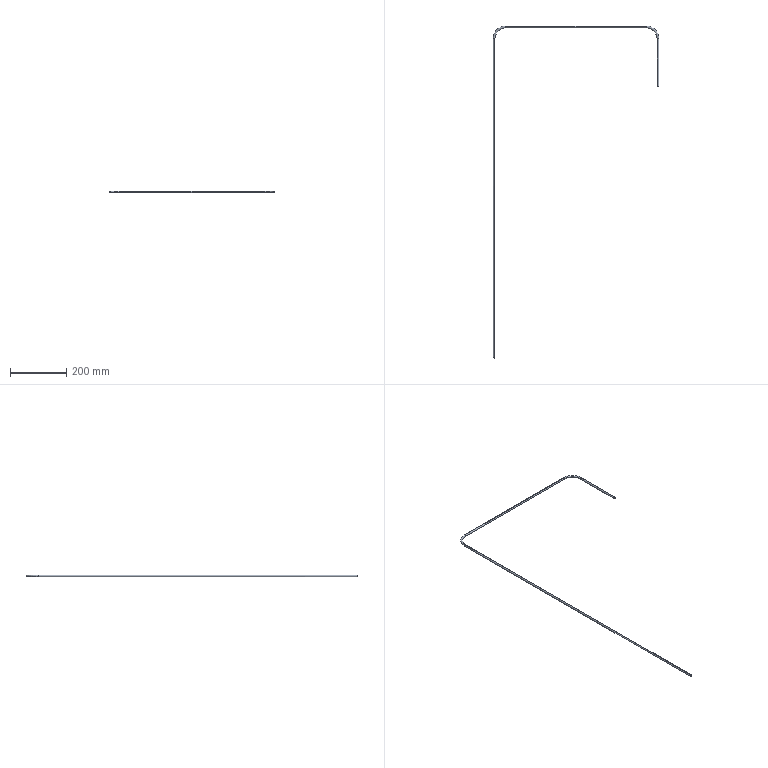Part | SolidWorks | features Sweep 1 | 1 solid | 12 faces | box 588.5 x 1178 x 6.5 mm | volume 64106 mm3 | cylinder 6 | torus 4 | plane 2 | commonest cylinder face diameters 6.5 x6
STEP:
#1=CARTESIAN_POINT('',(540.,1175.,-3.25));
#2=VERTEX_POINT('',#1);
#3=CARTESIAN_POINT('',(540.,1178.25,0.));
#4=VERTEX_POINT('',#3);
#5=CARTESIAN_POINT('',(540.,1175.,0.));
#6=DIRECTION('',(1.,0.,0.));
#7=DIRECTION('',(0.,0.,1.));
#8=AXIS2_PLACEMENT_3D('',#5,#6,#7);
#9=CIRCLE('',#8,3.25);
#10=EDGE_CURVE('',#2,#4,#9,.T.);
#11=ORIENTED_EDGE('',*,*,#10,.T.);
#12=CARTESIAN_POINT('',(585.25,1133.,0.));
#13=VERTEX_POINT('',#12);
#14=CARTESIAN_POINT('',(540.,1133.,0.));
#15=DIRECTION('',(0.,0.,-1.));
#16=DIRECTION('',(-1.,0.,0.));
#17=AXIS2_PLACEMENT_3D('',#14,#15,#16);
#18=CIRCLE('',#17,45.25);
#19=EDGE_CURVE('',#4,#13,#18,.T.);
#20=ORIENTED_EDGE('',*,*,#19,.T.);
#21=CARTESIAN_POINT('',(582.,1133.,-3.25));
#22=VERTEX_POINT('',#21);
#23=CARTESIAN_POINT('',(582.,1133.,0.));
#24=DIRECTION('',(0.,-1.,0.));
#25=DIRECTION('',(0.,0.,1.));
#26=AXIS2_PLACEMENT_3D('',#23,#24,#25);
#27=CIRCLE('',#26,3.25);
#28=EDGE_CURVE('',#22,#13,#27,.T.);
#29=ORIENTED_EDGE('',*,*,#28,.F.);
#30=CARTESIAN_POINT('',(578.75,1133.,0.));
#31=VERTEX_POINT('',#30);
#32=CARTESIAN_POINT('',(582.,1133.,0.));
#33=DIRECTION('',(0.,-1.,0.));
#34=DIRECTION('',(0.,0.,1.));
#35=AXIS2_PLACEMENT_3D('',#32,#33,#34);
#36=CIRCLE('',#35,3.25);
#37=EDGE_CURVE('',#31,#22,#36,.T.);
#38=ORIENTED_EDGE('',*,*,#37,.F.);
#39=CARTESIAN_POINT('',(540.,1171.75,0.));
#40=VERTEX_POINT('',#39);
#41=CARTESIAN_POINT('',(540.,1133.,0.));
#42=DIRECTION('',(0.,0.,-1.));
#43=DIRECTION('',(-1.,0.,0.));
#44=AXIS2_PLACEMENT_3D('',#41,#42,#43);
#45=CIRCLE('',#44,38.75);
#46=EDGE_CURVE('',#40,#31,#45,.T.);
#47=ORIENTED_EDGE('',*,*,#46,.F.);
#48=CARTESIAN_POINT('',(540.,1175.,0.));
#49=DIRECTION('',(1.,0.,0.));
#50=DIRECTION('',(0.,0.,1.));
#51=AXIS2_PLACEMENT_3D('',#48,#49,#50);
#52=CIRCLE('',#51,3.25);
#53=EDGE_CURVE('',#40,#2,#52,.T.);
#54=ORIENTED_EDGE('',*,*,#53,.T.);
#55=EDGE_LOOP('',(#11,#20,#29,#38,#47,#54));
#56=FACE_OUTER_BOUND('',#55,.T.);
#57=CARTESIAN_POINT('',(540.,1133.,0.));
#58=DIRECTION('',(0.,0.,-1.));
#59=DIRECTION('',(-1.,0.,0.));
#60=AXIS2_PLACEMENT_3D('',#57,#58,#59);
#61=TOROIDAL_SURFACE('',#60,42.,3.25);
#62=ADVANCED_FACE('',(#56),#61,.T.);
#63=CARTESIAN_POINT('',(0.,1133.,-3.25));
#64=VERTEX_POINT('',#63);
#65=CARTESIAN_POINT('',(-3.25,1133.,0.));
#66=VERTEX_POINT('',#65);
#67=CARTESIAN_POINT('',(0.,1133.,0.));
#68=DIRECTION('',(0.,1.,0.));
#69=DIRECTION('',(0.,0.,1.));
#70=AXIS2_PLACEMENT_3D('',#67,#68,#69);
#71=CIRCLE('',#70,3.25);
#72=EDGE_CURVE('',#64,#66,#71,.T.);
#73=ORIENTED_EDGE('',*,*,#72,.T.);
#74=CARTESIAN_POINT('',(42.,1178.25,0.));
#75=VERTEX_POINT('',#74);
#76=CARTESIAN_POINT('',(42.,1133.,0.));
#77=DIRECTION('',(0.,0.,-1.));
#78=DIRECTION('',(-1.,0.,0.));
#79=AXIS2_PLACEMENT_3D('',#76,#77,#78);
#80=CIRCLE('',#79,45.25);
#81=EDGE_CURVE('',#66,#75,#80,.T.);
#82=ORIENTED_EDGE('',*,*,#81,.T.);
#83=CARTESIAN_POINT('',(42.,1175.,-3.25));
#84=VERTEX_POINT('',#83);
#85=CARTESIAN_POINT('',(42.,1175.,0.));
#86=DIRECTION('',(1.,0.,0.));
#87=DIRECTION('',(0.,0.,1.));
#88=AXIS2_PLACEMENT_3D('',#85,#86,#87);
#89=CIRCLE('',#88,3.25);
#90=EDGE_CURVE('',#84,#75,#89,.T.);
#91=ORIENTED_EDGE('',*,*,#90,.F.);
#92=CARTESIAN_POINT('',(42.,1171.75,0.));
#93=VERTEX_POINT('',#92);
#94=CARTESIAN_POINT('',(42.,1175.,0.));
#95=DIRECTION('',(1.,0.,0.));
#96=DIRECTION('',(0.,0.,1.));
#97=AXIS2_PLACEMENT_3D('',#94,#95,#96);
#98=CIRCLE('',#97,3.25);
#99=EDGE_CURVE('',#93,#84,#98,.T.);
#100=ORIENTED_EDGE('',*,*,#99,.F.);
#101=CARTESIAN_POINT('',(3.25,1133.,0.));
#102=VERTEX_POINT('',#101);
#103=CARTESIAN_POINT('',(42.,1133.,0.));
#104=DIRECTION('',(0.,0.,-1.));
#105=DIRECTION('',(-1.,0.,0.));
#106=AXIS2_PLACEMENT_3D('',#103,#104,#105);
#107=CIRCLE('',#106,38.75);
#108=EDGE_CURVE('',#102,#93,#107,.T.);
#109=ORIENTED_EDGE('',*,*,#108,.F.);
#110=CARTESIAN_POINT('',(0.,1133.,0.));
#111=DIRECTION('',(0.,1.,0.));
#112=DIRECTION('',(0.,0.,1.));
#113=AXIS2_PLACEMENT_3D('',#110,#111,#112);
#114=CIRCLE('',#113,3.25);
#115=EDGE_CURVE('',#102,#64,#114,.T.);
#116=ORIENTED_EDGE('',*,*,#115,.T.);
#117=EDGE_LOOP('',(#73,#82,#91,#100,#109,#116));
#118=FACE_OUTER_BOUND('',#117,.T.);
#119=CARTESIAN_POINT('',(42.,1133.,0.));
#120=DIRECTION('',(0.,0.,-1.));
#121=DIRECTION('',(-1.,0.,0.));
#122=AXIS2_PLACEMENT_3D('',#119,#120,#121);
#123=TOROIDAL_SURFACE('',#122,42.,3.25);
#124=ADVANCED_FACE('',(#118),#123,.T.);
#125=ORIENTED_EDGE('',*,*,#28,.T.);
#126=CARTESIAN_POINT('',(582.,1133.,3.25));
#127=VERTEX_POINT('',#126);
#128=CARTESIAN_POINT('',(582.,1133.,0.));
#129=DIRECTION('',(0.,-1.,0.));
#130=DIRECTION('',(0.,0.,1.));
#131=AXIS2_PLACEMENT_3D('',#128,#129,#130);
#132=CIRCLE('',#131,3.25);
#133=EDGE_CURVE('',#13,#127,#132,.T.);
#134=ORIENTED_EDGE('',*,*,#133,.T.);
#135=CARTESIAN_POINT('',(582.,964.057,3.25));
#136=VERTEX_POINT('',#135);
#137=CARTESIAN_POINT('',(582.,1133.,3.25));
#138=DIRECTION('',(0.,-1.,0.));
#139=VECTOR('',#138,1000.);
#140=LINE('',#137,#139);
#141=EDGE_CURVE('',#127,#136,#140,.T.);
#142=ORIENTED_EDGE('',*,*,#141,.T.);
#143=CARTESIAN_POINT('',(582.,964.057,-3.25));
#144=VERTEX_POINT('',#143);
#145=CARTESIAN_POINT('',(582.,964.057,0.));
#146=DIRECTION('',(0.,-1.,0.));
#147=DIRECTION('',(0.,0.,1.));
#148=AXIS2_PLACEMENT_3D('',#145,#146,#147);
#149=CIRCLE('',#148,3.25);
#150=EDGE_CURVE('',#144,#136,#149,.T.);
#151=ORIENTED_EDGE('',*,*,#150,.F.);
#152=CARTESIAN_POINT('',(582.,1133.,-3.25));
#153=DIRECTION('',(0.,-1.,0.));
#154=VECTOR('',#153,1000.);
#155=LINE('',#152,#154);
#156=EDGE_CURVE('',#22,#144,#155,.T.);
#157=ORIENTED_EDGE('',*,*,#156,.F.);
#158=EDGE_LOOP('',(#125,#134,#142,#151,#157));
#159=FACE_OUTER_BOUND('',#158,.T.);
#160=CARTESIAN_POINT('',(582.,1133.,0.));
#161=DIRECTION('',(0.,-1.,0.));
#162=DIRECTION('',(0.,0.,-1.));
#163=AXIS2_PLACEMENT_3D('',#160,#161,#162);
#164=CYLINDRICAL_SURFACE('',#163,3.25);
#165=ADVANCED_FACE('',(#159),#164,.T.);
#166=ORIENTED_EDGE('',*,*,#90,.T.);
#167=CARTESIAN_POINT('',(42.,1175.,3.25));
#168=VERTEX_POINT('',#167);
#169=CARTESIAN_POINT('',(42.,1175.,0.));
#170=DIRECTION('',(1.,0.,0.));
#171=DIRECTION('',(0.,0.,1.));
#172=AXIS2_PLACEMENT_3D('',#169,#170,#171);
#173=CIRCLE('',#172,3.25);
#174=EDGE_CURVE('',#75,#168,#173,.T.);
#175=ORIENTED_EDGE('',*,*,#174,.T.);
#176=CARTESIAN_POINT('',(540.,1175.,3.25));
#177=VERTEX_POINT('',#176);
#178=CARTESIAN_POINT('',(42.,1175.,3.25));
#179=DIRECTION('',(1.,0.,0.));
#180=VECTOR('',#179,1000.);
#181=LINE('',#178,#180);
#182=EDGE_CURVE('',#168,#177,#181,.T.);
#183=ORIENTED_EDGE('',*,*,#182,.T.);
#184=CARTESIAN_POINT('',(540.,1175.,0.));
#185=DIRECTION('',(1.,0.,0.));
#186=DIRECTION('',(0.,0.,1.));
#187=AXIS2_PLACEMENT_3D('',#184,#185,#186);
#188=CIRCLE('',#187,3.25);
#189=EDGE_CURVE('',#4,#177,#188,.T.);
#190=ORIENTED_EDGE('',*,*,#189,.F.);
#191=ORIENTED_EDGE('',*,*,#10,.F.);
#192=CARTESIAN_POINT('',(42.,1175.,-3.25));
#193=DIRECTION('',(1.,0.,0.));
#194=VECTOR('',#193,1000.);
#195=LINE('',#192,#194);
#196=EDGE_CURVE('',#84,#2,#195,.T.);
#197=ORIENTED_EDGE('',*,*,#196,.F.);
#198=EDGE_LOOP('',(#166,#175,#183,#190,#191,#197));
#199=FACE_OUTER_BOUND('',#198,.T.);
#200=CARTESIAN_POINT('',(42.,1175.,0.));
#201=DIRECTION('',(1.,0.,0.));
#202=DIRECTION('',(0.,0.,-1.));
#203=AXIS2_PLACEMENT_3D('',#200,#201,#202);
#204=CYLINDRICAL_SURFACE('',#203,3.25);
#205=ADVANCED_FACE('',(#199),#204,.T.);
#206=CARTESIAN_POINT('',(0.,0.,3.25));
#207=VERTEX_POINT('',#206);
#208=CARTESIAN_POINT('',(0.,0.,-3.25));
#209=VERTEX_POINT('',#208);
#210=CARTESIAN_POINT('',(0.,0.,0.));
#211=DIRECTION('',(0.,1.,0.));
#212=DIRECTION('',(0.,0.,1.));
#213=AXIS2_PLACEMENT_3D('',#210,#211,#212);
#214=CIRCLE('',#213,3.25);
#215=EDGE_CURVE('',#207,#209,#214,.T.);
#216=ORIENTED_EDGE('',*,*,#215,.T.);
#217=CARTESIAN_POINT('',(0.,0.,-3.25));
#218=DIRECTION('',(0.,1.,0.));
#219=VECTOR('',#218,1000.);
#220=LINE('',#217,#219);
#221=EDGE_CURVE('',#209,#64,#220,.T.);
#222=ORIENTED_EDGE('',*,*,#221,.T.);
#223=ORIENTED_EDGE('',*,*,#115,.F.);
#224=CARTESIAN_POINT('',(0.,1133.,3.25));
#225=VERTEX_POINT('',#224);
#226=CARTESIAN_POINT('',(0.,1133.,0.));
#227=DIRECTION('',(0.,1.,0.));
#228=DIRECTION('',(0.,0.,1.));
#229=AXIS2_PLACEMENT_3D('',#226,#227,#228);
#230=CIRCLE('',#229,3.25);
#231=EDGE_CURVE('',#225,#102,#230,.T.);
#232=ORIENTED_EDGE('',*,*,#231,.F.);
#233=CARTESIAN_POINT('',(0.,0.,3.25));
#234=DIRECTION('',(0.,1.,0.));
#235=VECTOR('',#234,1000.);
#236=LINE('',#233,#235);
#237=EDGE_CURVE('',#207,#225,#236,.T.);
#238=ORIENTED_EDGE('',*,*,#237,.F.);
#239=EDGE_LOOP('',(#216,#222,#223,#232,#238));
#240=FACE_OUTER_BOUND('',#239,.T.);
#241=CARTESIAN_POINT('',(0.,0.,0.));
#242=DIRECTION('',(0.,1.,0.));
#243=DIRECTION('',(0.,0.,1.));
#244=AXIS2_PLACEMENT_3D('',#241,#242,#243);
#245=CYLINDRICAL_SURFACE('',#244,3.25);
#246=ADVANCED_FACE('',(#240),#245,.T.);
#247=ORIENTED_EDGE('',*,*,#141,.F.);
#248=CARTESIAN_POINT('',(582.,1133.,0.));
#249=DIRECTION('',(0.,-1.,0.));
#250=DIRECTION('',(0.,0.,1.));
#251=AXIS2_PLACEMENT_3D('',#248,#249,#250);
#252=CIRCLE('',#251,3.25);
#253=EDGE_CURVE('',#127,#31,#252,.T.);
#254=ORIENTED_EDGE('',*,*,#253,.T.);
#255=ORIENTED_EDGE('',*,*,#37,.T.);
#256=ORIENTED_EDGE('',*,*,#156,.T.);
#257=CARTESIAN_POINT('',(582.,964.057,0.));
#258=DIRECTION('',(0.,-1.,0.));
#259=DIRECTION('',(0.,0.,1.));
#260=AXIS2_PLACEMENT_3D('',#257,#258,#259);
#261=CIRCLE('',#260,3.25);
#262=EDGE_CURVE('',#136,#144,#261,.T.);
#263=ORIENTED_EDGE('',*,*,#262,.F.);
#264=EDGE_LOOP('',(#247,#254,#255,#256,#263));
#265=FACE_OUTER_BOUND('',#264,.T.);
#266=CARTESIAN_POINT('',(582.,1133.,0.));
#267=DIRECTION('',(0.,-1.,0.));
#268=DIRECTION('',(0.,0.,-1.));
#269=AXIS2_PLACEMENT_3D('',#266,#267,#268);
#270=CYLINDRICAL_SURFACE('',#269,3.25);
#271=ADVANCED_FACE('',(#265),#270,.T.);
#272=ORIENTED_EDGE('',*,*,#19,.F.);
#273=ORIENTED_EDGE('',*,*,#189,.T.);
#274=CARTESIAN_POINT('',(540.,1175.,0.));
#275=DIRECTION('',(1.,0.,0.));
#276=DIRECTION('',(0.,0.,1.));
#277=AXIS2_PLACEMENT_3D('',#274,#275,#276);
#278=CIRCLE('',#277,3.25);
#279=EDGE_CURVE('',#177,#40,#278,.T.);
#280=ORIENTED_EDGE('',*,*,#279,.T.);
#281=ORIENTED_EDGE('',*,*,#46,.T.);
#282=ORIENTED_EDGE('',*,*,#253,.F.);
#283=ORIENTED_EDGE('',*,*,#133,.F.);
#284=EDGE_LOOP('',(#272,#273,#280,#281,#282,#283));
#285=FACE_OUTER_BOUND('',#284,.T.);
#286=CARTESIAN_POINT('',(540.,1133.,0.));
#287=DIRECTION('',(0.,0.,-1.));
#288=DIRECTION('',(-1.,0.,0.));
#289=AXIS2_PLACEMENT_3D('',#286,#287,#288);
#290=TOROIDAL_SURFACE('',#289,42.,3.25);
#291=ADVANCED_FACE('',(#285),#290,.T.);
#292=ORIENTED_EDGE('',*,*,#182,.F.);
#293=CARTESIAN_POINT('',(42.,1175.,0.));
#294=DIRECTION('',(1.,0.,0.));
#295=DIRECTION('',(0.,0.,1.));
#296=AXIS2_PLACEMENT_3D('',#293,#294,#295);
#297=CIRCLE('',#296,3.25);
#298=EDGE_CURVE('',#168,#93,#297,.T.);
#299=ORIENTED_EDGE('',*,*,#298,.T.);
#300=ORIENTED_EDGE('',*,*,#99,.T.);
#301=ORIENTED_EDGE('',*,*,#196,.T.);
#302=ORIENTED_EDGE('',*,*,#53,.F.);
#303=ORIENTED_EDGE('',*,*,#279,.F.);
#304=EDGE_LOOP('',(#292,#299,#300,#301,#302,#303));
#305=FACE_OUTER_BOUND('',#304,.T.);
#306=CARTESIAN_POINT('',(42.,1175.,0.));
#307=DIRECTION('',(1.,0.,0.));
#308=DIRECTION('',(0.,0.,-1.));
#309=AXIS2_PLACEMENT_3D('',#306,#307,#308);
#310=CYLINDRICAL_SURFACE('',#309,3.25);
#311=ADVANCED_FACE('',(#305),#310,.T.);
#312=ORIENTED_EDGE('',*,*,#81,.F.);
#313=CARTESIAN_POINT('',(0.,1133.,0.));
#314=DIRECTION('',(0.,1.,0.));
#315=DIRECTION('',(0.,0.,1.));
#316=AXIS2_PLACEMENT_3D('',#313,#314,#315);
#317=CIRCLE('',#316,3.25);
#318=EDGE_CURVE('',#66,#225,#317,.T.);
#319=ORIENTED_EDGE('',*,*,#318,.T.);
#320=ORIENTED_EDGE('',*,*,#231,.T.);
#321=ORIENTED_EDGE('',*,*,#108,.T.);
#322=ORIENTED_EDGE('',*,*,#298,.F.);
#323=ORIENTED_EDGE('',*,*,#174,.F.);
#324=EDGE_LOOP('',(#312,#319,#320,#321,#322,#323));
#325=FACE_OUTER_BOUND('',#324,.T.);
#326=CARTESIAN_POINT('',(42.,1133.,0.));
#327=DIRECTION('',(0.,0.,-1.));
#328=DIRECTION('',(-1.,0.,0.));
#329=AXIS2_PLACEMENT_3D('',#326,#327,#328);
#330=TOROIDAL_SURFACE('',#329,42.,3.25);
#331=ADVANCED_FACE('',(#325),#330,.T.);
#332=ORIENTED_EDGE('',*,*,#221,.F.);
#333=CARTESIAN_POINT('',(0.,0.,0.));
#334=DIRECTION('',(0.,1.,0.));
#335=DIRECTION('',(0.,0.,1.));
#336=AXIS2_PLACEMENT_3D('',#333,#334,#335);
#337=CIRCLE('',#336,3.25);
#338=EDGE_CURVE('',#209,#207,#337,.T.);
#339=ORIENTED_EDGE('',*,*,#338,.T.);
#340=ORIENTED_EDGE('',*,*,#237,.T.);
#341=ORIENTED_EDGE('',*,*,#318,.F.);
#342=ORIENTED_EDGE('',*,*,#72,.F.);
#343=EDGE_LOOP('',(#332,#339,#340,#341,#342));
#344=FACE_OUTER_BOUND('',#343,.T.);
#345=CARTESIAN_POINT('',(0.,0.,0.));
#346=DIRECTION('',(0.,1.,0.));
#347=DIRECTION('',(0.,0.,1.));
#348=AXIS2_PLACEMENT_3D('',#345,#346,#347);
#349=CYLINDRICAL_SURFACE('',#348,3.25);
#350=ADVANCED_FACE('',(#344),#349,.T.);
#351=ORIENTED_EDGE('',*,*,#150,.T.);
#352=ORIENTED_EDGE('',*,*,#262,.T.);
#353=EDGE_LOOP('',(#351,#352));
#354=FACE_OUTER_BOUND('',#353,.T.);
#355=CARTESIAN_POINT('',(582.,964.057,0.));
#356=DIRECTION('',(0.,-1.,0.));
#357=DIRECTION('',(0.,0.,1.));
#358=AXIS2_PLACEMENT_3D('',#355,#356,#357);
#359=PLANE('',#358);
#360=ADVANCED_FACE('',(#354),#359,.T.);
#361=ORIENTED_EDGE('',*,*,#215,.F.);
#362=ORIENTED_EDGE('',*,*,#338,.F.);
#363=EDGE_LOOP('',(#361,#362));
#364=FACE_OUTER_BOUND('',#363,.T.);
#365=CARTESIAN_POINT('',(0.,0.,0.));
#366=DIRECTION('',(0.,1.,0.));
#367=DIRECTION('',(0.,0.,1.));
#368=AXIS2_PLACEMENT_3D('',#365,#366,#367);
#369=PLANE('',#368);
#370=ADVANCED_FACE('',(#364),#369,.F.);
#371=CLOSED_SHELL('',(#62,#124,#165,#205,#246,#271,#291,#311,#331,#350,#360,#370));
#372=MANIFOLD_SOLID_BREP('',#371);
#373=CARTESIAN_POINT('',(0.,0.,0.));
#374=DIRECTION('',(0.,0.,1.));
#375=DIRECTION('',(1.,0.,0.));
#376=AXIS2_PLACEMENT_3D('',#373,#374,#375);
#377=(LENGTH_UNIT()NAMED_UNIT(*)SI_UNIT(.MILLI.,.METRE.));
#378=UNCERTAINTY_MEASURE_WITH_UNIT(LENGTH_MEASURE(0.00001),#377,'','');
#379=(NAMED_UNIT(*)PLANE_ANGLE_UNIT()SI_UNIT($,.RADIAN.));
#380=(NAMED_UNIT(*)SI_UNIT($,.STERADIAN.)SOLID_ANGLE_UNIT());
#381=(GEOMETRIC_REPRESENTATION_CONTEXT(3)GLOBAL_UNCERTAINTY_ASSIGNED_CONTEXT((#378))GLOBAL_UNIT_ASSIGNED_CONTEXT((#377,#379,#380))REPRESENTATION_CONTEXT('',''));
#382=ADVANCED_BREP_SHAPE_REPRESENTATION('',(#372,#376),#381);